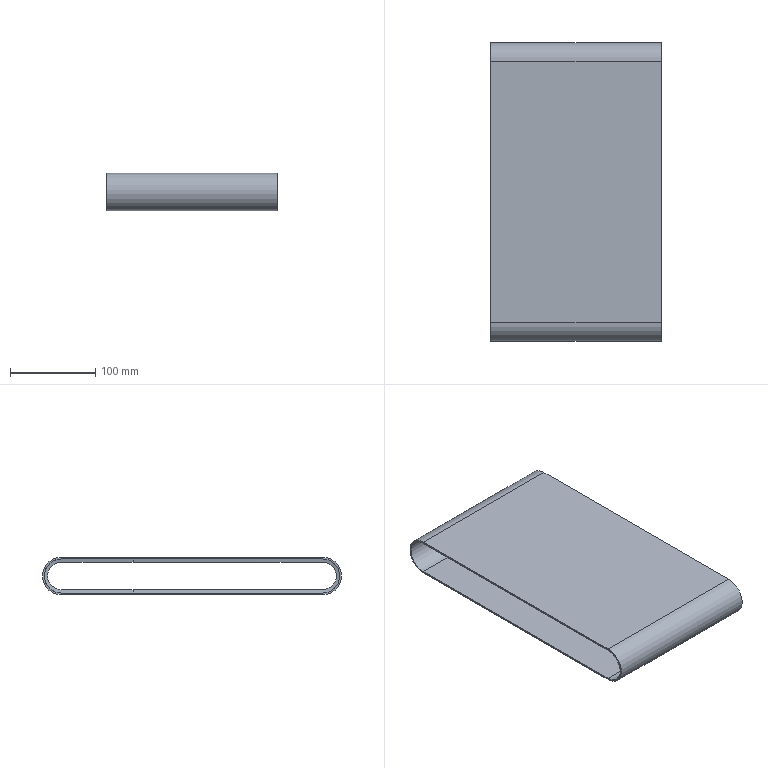Part | STEP file | YBQDJ-SSJ-3 | 1 solid | 20 faces | box 200 x 350 x 44 mm | volume 311989 mm3 | plane 8 | cylinder 6 | spline 6 | commonest cylinder face diameters 40 x4 44 x2